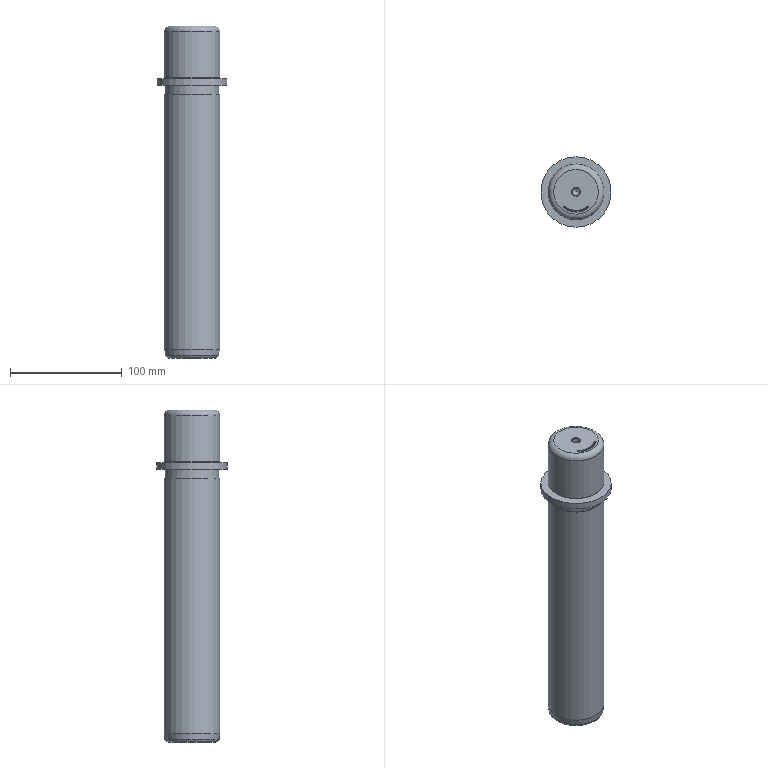Part | NX | features 1 2 | 1 solid | 301 faces | box 63 x 63 x 297 mm | volume 585349 mm3 | spline 174 | plane 114 | cylinder 7 | cone 4 | torus 2 | commonest cylinder face diameters 6.647 x2 48 x2 50 x2 63 x1